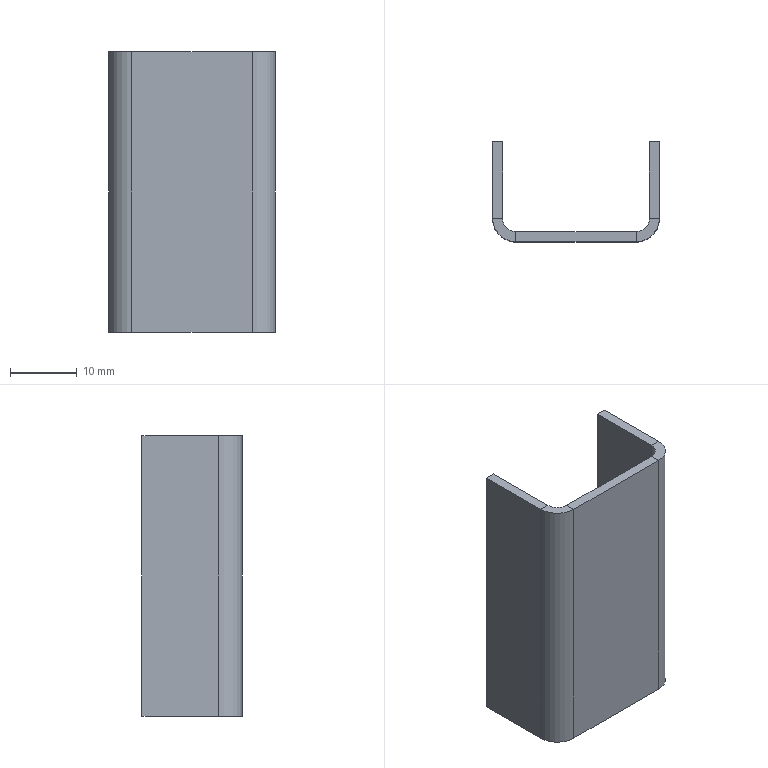Part | STEP file | Reinforcing rib 1001 | 1 solid | 22 faces | box 25 x 15 x 42 mm | volume 3127 mm3 | plane 18 | cylinder 4 | commonest cylinder face diameters 4 x2 7 x2
STEP:
#1=CARTESIAN_POINT('',(0.,0.,0.));
#2=DIRECTION('',(0.,0.,1.));
#3=DIRECTION('',(1.,0.,0.));
#4=AXIS2_PLACEMENT_3D('',#1,#2,#3);
#5=CARTESIAN_POINT('',(-12.5,3.5,21.));
#6=VERTEX_POINT('',#5);
#7=CARTESIAN_POINT('',(-11.,3.5,21.));
#8=VERTEX_POINT('',#7);
#9=CARTESIAN_POINT('',(-12.5,3.5,21.));
#10=DIRECTION('',(1.,0.,0.));
#11=VECTOR('',#10,1.);
#12=LINE('',#9,#11);
#13=CARTESIAN_POINT('',(-12.5,3.5,21.));
#14=DIRECTION('',(0.,0.,1.));
#15=DIRECTION('',(1.,0.,0.));
#16=AXIS2_PLACEMENT_3D('',#13,#14,#15);
#17=PLANE('',#16);
#18=CARTESIAN_POINT('',(0.,0.));
#19=DIRECTION('',(1.,0.));
#20=VECTOR('',#19,1.);
#21=LINE('',#18,#20);
#22=(GEOMETRIC_REPRESENTATION_CONTEXT(2)PARAMETRIC_REPRESENTATION_CONTEXT()REPRESENTATION_CONTEXT('',''));
#23=DEFINITIONAL_REPRESENTATION('',(#21),#22);
#24=PCURVE('',#17,#23);
#25=CARTESIAN_POINT('',(-9.,1.5,21.));
#26=DIRECTION('',(0.,0.,1.));
#27=DIRECTION('',(1.,0.,0.));
#28=AXIS2_PLACEMENT_3D('',#25,#26,#27);
#29=PLANE('',#28);
#30=CARTESIAN_POINT('',(-3.5,2.));
#31=DIRECTION('',(1.,0.));
#32=VECTOR('',#31,1.);
#33=LINE('',#30,#32);
#34=(GEOMETRIC_REPRESENTATION_CONTEXT(2)PARAMETRIC_REPRESENTATION_CONTEXT()REPRESENTATION_CONTEXT('',''));
#35=DEFINITIONAL_REPRESENTATION('',(#33),#34);
#36=PCURVE('',#29,#35);
#37=SURFACE_CURVE('',#12,(#24,#36),.PCURVE_S1.);
#38=EDGE_CURVE('',#6,#8,#37,.T.);
#39=ORIENTED_EDGE('',*,*,#38,.F.);
#40=CARTESIAN_POINT('',(-9.,0.,21.));
#41=VERTEX_POINT('',#40);
#42=CARTESIAN_POINT('',(-9.,3.5,21.));
#43=DIRECTION('',(0.,0.,1.));
#44=DIRECTION('',(-1.,0.,0.));
#45=AXIS2_PLACEMENT_3D('',#42,#43,#44);
#46=CIRCLE('',#45,3.5);
#47=CARTESIAN_POINT('',(3.5,0.));
#48=DIRECTION('',(-1.,0.));
#49=AXIS2_PLACEMENT_2D('',#47,#48);
#50=CIRCLE('',#49,3.5);
#51=(GEOMETRIC_REPRESENTATION_CONTEXT(2)PARAMETRIC_REPRESENTATION_CONTEXT()REPRESENTATION_CONTEXT('',''));
#52=DEFINITIONAL_REPRESENTATION('',(#50),#51);
#53=PCURVE('',#17,#52);
#54=CARTESIAN_POINT('',(-9.,3.5,21.));
#55=DIRECTION('',(0.,0.,-1.));
#56=DIRECTION('',(-1.,0.,0.));
#57=AXIS2_PLACEMENT_3D('',#54,#55,#56);
#58=CYLINDRICAL_SURFACE('',#57,3.5);
#59=CARTESIAN_POINT('',(6.283,0.));
#60=DIRECTION('',(-1.,0.));
#61=VECTOR('',#60,1.);
#62=LINE('',#59,#61);
#63=(GEOMETRIC_REPRESENTATION_CONTEXT(2)PARAMETRIC_REPRESENTATION_CONTEXT()REPRESENTATION_CONTEXT('',''));
#64=DEFINITIONAL_REPRESENTATION('',(#62),#63);
#65=PCURVE('',#58,#64);
#66=SURFACE_CURVE('',#46,(#53,#65),.PCURVE_S1.);
#67=EDGE_CURVE('',#6,#41,#66,.T.);
#68=ORIENTED_EDGE('',*,*,#67,.T.);
#69=CARTESIAN_POINT('',(-9.,1.5,21.));
#70=VERTEX_POINT('',#69);
#71=CARTESIAN_POINT('',(-9.,1.5,21.));
#72=DIRECTION('',(0.,-1.,0.));
#73=VECTOR('',#72,1.);
#74=LINE('',#71,#73);
#75=CARTESIAN_POINT('',(3.5,-2.));
#76=DIRECTION('',(0.,-1.));
#77=VECTOR('',#76,1.);
#78=LINE('',#75,#77);
#79=(GEOMETRIC_REPRESENTATION_CONTEXT(2)PARAMETRIC_REPRESENTATION_CONTEXT()REPRESENTATION_CONTEXT('',''));
#80=DEFINITIONAL_REPRESENTATION('',(#78),#79);
#81=PCURVE('',#17,#80);
#82=CARTESIAN_POINT('',(11.,3.5,21.));
#83=DIRECTION('',(0.,0.,1.));
#84=DIRECTION('',(1.,0.,0.));
#85=AXIS2_PLACEMENT_3D('',#82,#83,#84);
#86=PLANE('',#85);
#87=CARTESIAN_POINT('',(-20.,-2.));
#88=DIRECTION('',(0.,-1.));
#89=VECTOR('',#88,1.);
#90=LINE('',#87,#89);
#91=(GEOMETRIC_REPRESENTATION_CONTEXT(2)PARAMETRIC_REPRESENTATION_CONTEXT()REPRESENTATION_CONTEXT('',''));
#92=DEFINITIONAL_REPRESENTATION('',(#90),#91);
#93=PCURVE('',#86,#92);
#94=SURFACE_CURVE('',#74,(#81,#93),.PCURVE_S1.);
#95=EDGE_CURVE('',#70,#41,#94,.T.);
#96=ORIENTED_EDGE('',*,*,#95,.F.);
#97=CARTESIAN_POINT('',(-9.,3.5,21.));
#98=DIRECTION('',(0.,0.,1.));
#99=DIRECTION('',(1.,0.,0.));
#100=AXIS2_PLACEMENT_3D('',#97,#98,#99);
#101=CIRCLE('',#100,2.);
#102=CARTESIAN_POINT('',(3.5,0.));
#103=DIRECTION('',(1.,0.));
#104=AXIS2_PLACEMENT_2D('',#102,#103);
#105=CIRCLE('',#104,2.);
#106=(GEOMETRIC_REPRESENTATION_CONTEXT(2)PARAMETRIC_REPRESENTATION_CONTEXT()REPRESENTATION_CONTEXT('',''));
#107=DEFINITIONAL_REPRESENTATION('',(#105),#106);
#108=PCURVE('',#17,#107);
#109=CARTESIAN_POINT('',(-9.,3.5,21.));
#110=DIRECTION('',(0.,0.,-1.));
#111=DIRECTION('',(-1.,0.,0.));
#112=AXIS2_PLACEMENT_3D('',#109,#110,#111);
#113=CYLINDRICAL_SURFACE('',#112,2.);
#114=CARTESIAN_POINT('',(9.425,0.));
#115=DIRECTION('',(-1.,0.));
#116=VECTOR('',#115,1.);
#117=LINE('',#114,#116);
#118=(GEOMETRIC_REPRESENTATION_CONTEXT(2)PARAMETRIC_REPRESENTATION_CONTEXT()REPRESENTATION_CONTEXT('',''));
#119=DEFINITIONAL_REPRESENTATION('',(#117),#118);
#120=PCURVE('',#113,#119);
#121=SURFACE_CURVE('',#101,(#108,#120),.PCURVE_S1.);
#122=EDGE_CURVE('',#8,#70,#121,.T.);
#123=ORIENTED_EDGE('',*,*,#122,.F.);
#124=EDGE_LOOP('',(#39,#68,#96,#123));
#125=FACE_BOUND('',#124,.T.);
#126=ADVANCED_FACE('',(#125),#17,.T.);
#127=CARTESIAN_POINT('',(-12.5,15.,21.));
#128=VERTEX_POINT('',#127);
#129=CARTESIAN_POINT('',(-12.5,15.,21.));
#130=DIRECTION('',(0.,-1.,0.));
#131=VECTOR('',#130,1.);
#132=LINE('',#129,#131);
#133=CARTESIAN_POINT('',(-3.5,13.5));
#134=DIRECTION('',(0.,-1.));
#135=VECTOR('',#134,1.);
#136=LINE('',#133,#135);
#137=(GEOMETRIC_REPRESENTATION_CONTEXT(2)PARAMETRIC_REPRESENTATION_CONTEXT()REPRESENTATION_CONTEXT('',''));
#138=DEFINITIONAL_REPRESENTATION('',(#136),#137);
#139=PCURVE('',#29,#138);
#140=CARTESIAN_POINT('',(-12.5,15.,21.));
#141=DIRECTION('',(1.,0.,0.));
#142=DIRECTION('',(0.,1.,0.));
#143=AXIS2_PLACEMENT_3D('',#140,#141,#142);
#144=PLANE('',#143);
#145=CARTESIAN_POINT('',(0.,0.));
#146=DIRECTION('',(-1.,0.));
#147=VECTOR('',#146,1.);
#148=LINE('',#145,#147);
#149=(GEOMETRIC_REPRESENTATION_CONTEXT(2)PARAMETRIC_REPRESENTATION_CONTEXT()REPRESENTATION_CONTEXT('',''));
#150=DEFINITIONAL_REPRESENTATION('',(#148),#149);
#151=PCURVE('',#144,#150);
#152=SURFACE_CURVE('',#132,(#139,#151),.PCURVE_S1.);
#153=EDGE_CURVE('',#128,#6,#152,.T.);
#154=ORIENTED_EDGE('',*,*,#153,.T.);
#155=ORIENTED_EDGE('',*,*,#38,.T.);
#156=CARTESIAN_POINT('',(-11.,15.,21.));
#157=VERTEX_POINT('',#156);
#158=CARTESIAN_POINT('',(-11.,15.,21.));
#159=DIRECTION('',(0.,-1.,0.));
#160=VECTOR('',#159,1.);
#161=LINE('',#158,#160);
#162=CARTESIAN_POINT('',(-2.,13.5));
#163=DIRECTION('',(0.,-1.));
#164=VECTOR('',#163,1.);
#165=LINE('',#162,#164);
#166=(GEOMETRIC_REPRESENTATION_CONTEXT(2)PARAMETRIC_REPRESENTATION_CONTEXT()REPRESENTATION_CONTEXT('',''));
#167=DEFINITIONAL_REPRESENTATION('',(#165),#166);
#168=PCURVE('',#29,#167);
#169=CARTESIAN_POINT('',(-11.,15.,21.));
#170=DIRECTION('',(1.,0.,0.));
#171=DIRECTION('',(0.,1.,0.));
#172=AXIS2_PLACEMENT_3D('',#169,#170,#171);
#173=PLANE('',#172);
#174=CARTESIAN_POINT('',(0.,0.));
#175=DIRECTION('',(-1.,0.));
#176=VECTOR('',#175,1.);
#177=LINE('',#174,#176);
#178=(GEOMETRIC_REPRESENTATION_CONTEXT(2)PARAMETRIC_REPRESENTATION_CONTEXT()REPRESENTATION_CONTEXT('',''));
#179=DEFINITIONAL_REPRESENTATION('',(#177),#178);
#180=PCURVE('',#173,#179);
#181=SURFACE_CURVE('',#161,(#168,#180),.PCURVE_S1.);
#182=EDGE_CURVE('',#157,#8,#181,.T.);
#183=ORIENTED_EDGE('',*,*,#182,.F.);
#184=CARTESIAN_POINT('',(-12.5,15.,21.));
#185=DIRECTION('',(1.,0.,0.));
#186=VECTOR('',#185,1.);
#187=LINE('',#184,#186);
#188=CARTESIAN_POINT('',(-3.5,13.5));
#189=DIRECTION('',(1.,0.));
#190=VECTOR('',#189,1.);
#191=LINE('',#188,#190);
#192=(GEOMETRIC_REPRESENTATION_CONTEXT(2)PARAMETRIC_REPRESENTATION_CONTEXT()REPRESENTATION_CONTEXT('',''));
#193=DEFINITIONAL_REPRESENTATION('',(#191),#192);
#194=PCURVE('',#29,#193);
#195=CARTESIAN_POINT('',(-12.5,15.,21.));
#196=DIRECTION('',(0.,1.,0.));
#197=DIRECTION('',(0.,0.,1.));
#198=AXIS2_PLACEMENT_3D('',#195,#196,#197);
#199=PLANE('',#198);
#200=CARTESIAN_POINT('',(0.,0.));
#201=DIRECTION('',(0.,1.));
#202=VECTOR('',#201,1.);
#203=LINE('',#200,#202);
#204=(GEOMETRIC_REPRESENTATION_CONTEXT(2)PARAMETRIC_REPRESENTATION_CONTEXT()REPRESENTATION_CONTEXT('',''));
#205=DEFINITIONAL_REPRESENTATION('',(#203),#204);
#206=PCURVE('',#199,#205);
#207=SURFACE_CURVE('',#187,(#194,#206),.PCURVE_S1.);
#208=EDGE_CURVE('',#128,#157,#207,.T.);
#209=ORIENTED_EDGE('',*,*,#208,.F.);
#210=EDGE_LOOP('',(#154,#155,#183,#209));
#211=FACE_BOUND('',#210,.T.);
#212=ADVANCED_FACE('',(#211),#29,.T.);
#213=CARTESIAN_POINT('',(-9.,0.,-21.));
#214=VERTEX_POINT('',#213);
#215=CARTESIAN_POINT('',(-9.,1.5,-21.));
#216=VERTEX_POINT('',#215);
#217=CARTESIAN_POINT('',(-9.,0.,-21.));
#218=DIRECTION('',(0.,1.,0.));
#219=VECTOR('',#218,1.);
#220=LINE('',#217,#219);
#221=CARTESIAN_POINT('',(-9.,0.,-21.));
#222=DIRECTION('',(0.,0.,-1.));
#223=DIRECTION('',(-1.,0.,0.));
#224=AXIS2_PLACEMENT_3D('',#221,#222,#223);
#225=PLANE('',#224);
#226=CARTESIAN_POINT('',(0.,0.));
#227=DIRECTION('',(0.,1.));
#228=VECTOR('',#227,1.);
#229=LINE('',#226,#228);
#230=(GEOMETRIC_REPRESENTATION_CONTEXT(2)PARAMETRIC_REPRESENTATION_CONTEXT()REPRESENTATION_CONTEXT('',''));
#231=DEFINITIONAL_REPRESENTATION('',(#229),#230);
#232=PCURVE('',#225,#231);
#233=CARTESIAN_POINT('',(-11.,3.5,-21.));
#234=DIRECTION('',(0.,0.,-1.));
#235=DIRECTION('',(-1.,0.,0.));
#236=AXIS2_PLACEMENT_3D('',#233,#234,#235);
#237=PLANE('',#236);
#238=CARTESIAN_POINT('',(-2.,-3.5));
#239=DIRECTION('',(0.,1.));
#240=VECTOR('',#239,1.);
#241=LINE('',#238,#240);
#242=(GEOMETRIC_REPRESENTATION_CONTEXT(2)PARAMETRIC_REPRESENTATION_CONTEXT()REPRESENTATION_CONTEXT('',''));
#243=DEFINITIONAL_REPRESENTATION('',(#241),#242);
#244=PCURVE('',#237,#243);
#245=SURFACE_CURVE('',#220,(#232,#244),.PCURVE_S1.);
#246=EDGE_CURVE('',#214,#216,#245,.T.);
#247=ORIENTED_EDGE('',*,*,#246,.F.);
#248=CARTESIAN_POINT('',(-12.5,3.5,-21.));
#249=VERTEX_POINT('',#248);
#250=CARTESIAN_POINT('',(-9.,3.5,-21.));
#251=DIRECTION('',(0.,0.,1.));
#252=DIRECTION('',(-1.,0.,0.));
#253=AXIS2_PLACEMENT_3D('',#250,#251,#252);
#254=CIRCLE('',#253,3.5);
#255=CARTESIAN_POINT('',(3.5,3.5));
#256=CARTESIAN_POINT('',(3.5,-2.562));
#257=CARTESIAN_POINT('',(-1.75,0.4689));
#258=CARTESIAN_POINT('',(-7.,3.5));
#259=CARTESIAN_POINT('',(-1.75,6.531));
#260=CARTESIAN_POINT('',(3.5,9.562));
#261=CARTESIAN_POINT('',(3.5,3.5));
#262=(BOUNDED_CURVE()B_SPLINE_CURVE(2,(#255,#256,#257,#258,#259,#260,#261),.UNSPECIFIED.,.T.,.F.)B_SPLINE_CURVE_WITH_KNOTS((1,2,2,2,2,1),(-2.094,0.,2.094,4.189,6.283,8.378),.UNSPECIFIED.)CURVE()GEOMETRIC_REPRESENTATION_ITEM()RATIONAL_B_SPLINE_CURVE((1.,0.5,1.,0.5,1.,0.5,1.))REPRESENTATION_ITEM(''));
#263=(GEOMETRIC_REPRESENTATION_CONTEXT(2)PARAMETRIC_REPRESENTATION_CONTEXT()REPRESENTATION_CONTEXT('',''));
#264=DEFINITIONAL_REPRESENTATION('',(#262),#263);
#265=PCURVE('',#225,#264);
#266=CARTESIAN_POINT('',(6.283,42.));
#267=DIRECTION('',(-1.,0.));
#268=VECTOR('',#267,1.);
#269=LINE('',#266,#268);
#270=(GEOMETRIC_REPRESENTATION_CONTEXT(2)PARAMETRIC_REPRESENTATION_CONTEXT()REPRESENTATION_CONTEXT('',''));
#271=DEFINITIONAL_REPRESENTATION('',(#269),#270);
#272=PCURVE('',#58,#271);
#273=SURFACE_CURVE('',#254,(#265,#272),.PCURVE_S1.);
#274=EDGE_CURVE('',#249,#214,#273,.T.);
#275=ORIENTED_EDGE('',*,*,#274,.F.);
#276=CARTESIAN_POINT('',(-11.,3.5,-21.));
#277=VERTEX_POINT('',#276);
#278=CARTESIAN_POINT('',(-11.,3.5,-21.));
#279=DIRECTION('',(-1.,0.,0.));
#280=VECTOR('',#279,1.);
#281=LINE('',#278,#280);
#282=CARTESIAN_POINT('',(2.,3.5));
#283=DIRECTION('',(1.,0.));
#284=VECTOR('',#283,1.);
#285=LINE('',#282,#284);
#286=(GEOMETRIC_REPRESENTATION_CONTEXT(2)PARAMETRIC_REPRESENTATION_CONTEXT()REPRESENTATION_CONTEXT('',''));
#287=DEFINITIONAL_REPRESENTATION('',(#285),#286);
#288=PCURVE('',#225,#287);
#289=CARTESIAN_POINT('',(9.,3.5,-21.));
#290=DIRECTION('',(0.,0.,1.));
#291=DIRECTION('',(1.,0.,0.));
#292=AXIS2_PLACEMENT_3D('',#289,#290,#291);
#293=PLANE('',#292);
#294=CARTESIAN_POINT('',(-20.,0.));
#295=DIRECTION('',(-1.,0.));
#296=VECTOR('',#295,1.);
#297=LINE('',#294,#296);
#298=(GEOMETRIC_REPRESENTATION_CONTEXT(2)PARAMETRIC_REPRESENTATION_CONTEXT()REPRESENTATION_CONTEXT('',''));
#299=DEFINITIONAL_REPRESENTATION('',(#297),#298);
#300=PCURVE('',#293,#299);
#301=SURFACE_CURVE('',#281,(#288,#300),.PCURVE_S1.);
#302=EDGE_CURVE('',#277,#249,#301,.T.);
#303=ORIENTED_EDGE('',*,*,#302,.F.);
#304=CARTESIAN_POINT('',(-9.,3.5,-21.));
#305=DIRECTION('',(0.,0.,1.));
#306=DIRECTION('',(1.,0.,0.));
#307=AXIS2_PLACEMENT_3D('',#304,#305,#306);
#308=CIRCLE('',#307,2.);
#309=CARTESIAN_POINT('',(-2.,3.5));
#310=CARTESIAN_POINT('',(-2.,6.964));
#311=CARTESIAN_POINT('',(1.,5.232));
#312=CARTESIAN_POINT('',(4.,3.5));
#313=CARTESIAN_POINT('',(1.,1.768));
#314=CARTESIAN_POINT('',(-2.,0.0359));
#315=CARTESIAN_POINT('',(-2.,3.5));
#316=(BOUNDED_CURVE()B_SPLINE_CURVE(2,(#309,#310,#311,#312,#313,#314,#315),.UNSPECIFIED.,.T.,.F.)B_SPLINE_CURVE_WITH_KNOTS((1,2,2,2,2,1),(-2.094,0.,2.094,4.189,6.283,8.378),.UNSPECIFIED.)CURVE()GEOMETRIC_REPRESENTATION_ITEM()RATIONAL_B_SPLINE_CURVE((1.,0.5,1.,0.5,1.,0.5,1.))REPRESENTATION_ITEM(''));
#317=(GEOMETRIC_REPRESENTATION_CONTEXT(2)PARAMETRIC_REPRESENTATION_CONTEXT()REPRESENTATION_CONTEXT('',''));
#318=DEFINITIONAL_REPRESENTATION('',(#316),#317);
#319=PCURVE('',#225,#318);
#320=CARTESIAN_POINT('',(9.425,42.));
#321=DIRECTION('',(-1.,0.));
#322=VECTOR('',#321,1.);
#323=LINE('',#320,#322);
#324=(GEOMETRIC_REPRESENTATION_CONTEXT(2)PARAMETRIC_REPRESENTATION_CONTEXT()REPRESENTATION_CONTEXT('',''));
#325=DEFINITIONAL_REPRESENTATION('',(#323),#324);
#326=PCURVE('',#113,#325);
#327=SURFACE_CURVE('',#308,(#319,#326),.PCURVE_S1.);
#328=EDGE_CURVE('',#277,#216,#327,.T.);
#329=ORIENTED_EDGE('',*,*,#328,.T.);
#330=EDGE_LOOP('',(#247,#275,#303,#329));
#331=FACE_BOUND('',#330,.T.);
#332=ADVANCED_FACE('',(#331),#225,.T.);
#333=CARTESIAN_POINT('',(9.,0.,-21.));
#334=VERTEX_POINT('',#333);
#335=CARTESIAN_POINT('',(-12.5,0.,-21.));
#336=DIRECTION('',(1.,0.,0.));
#337=VECTOR('',#336,1.);
#338=LINE('',#335,#337);
#339=CARTESIAN_POINT('',(1.5,-3.5));
#340=DIRECTION('',(-1.,0.));
#341=VECTOR('',#340,1.);
#342=LINE('',#339,#341);
#343=(GEOMETRIC_REPRESENTATION_CONTEXT(2)PARAMETRIC_REPRESENTATION_CONTEXT()REPRESENTATION_CONTEXT('',''));
#344=DEFINITIONAL_REPRESENTATION('',(#342),#343);
#345=PCURVE('',#237,#344);
#346=CARTESIAN_POINT('',(-12.5,0.,21.));
#347=DIRECTION('',(0.,1.,0.));
#348=DIRECTION('',(0.,0.,1.));
#349=AXIS2_PLACEMENT_3D('',#346,#347,#348);
#350=PLANE('',#349);
#351=CARTESIAN_POINT('',(-42.,0.));
#352=DIRECTION('',(0.,1.));
#353=VECTOR('',#352,1.);
#354=LINE('',#351,#353);
#355=(GEOMETRIC_REPRESENTATION_CONTEXT(2)PARAMETRIC_REPRESENTATION_CONTEXT()REPRESENTATION_CONTEXT('',''));
#356=DEFINITIONAL_REPRESENTATION('',(#354),#355);
#357=PCURVE('',#350,#356);
#358=SURFACE_CURVE('',#338,(#345,#357),.PCURVE_S1.);
#359=EDGE_CURVE('',#214,#334,#358,.T.);
#360=ORIENTED_EDGE('',*,*,#359,.F.);
#361=ORIENTED_EDGE('',*,*,#246,.T.);
#362=CARTESIAN_POINT('',(9.,1.5,-21.));
#363=VERTEX_POINT('',#362);
#364=CARTESIAN_POINT('',(-12.5,1.5,-21.));
#365=DIRECTION('',(1.,0.,0.));
#366=VECTOR('',#365,1.);
#367=LINE('',#364,#366);
#368=CARTESIAN_POINT('',(1.5,-2.));
#369=DIRECTION('',(-1.,0.));
#370=VECTOR('',#369,1.);
#371=LINE('',#368,#370);
#372=(GEOMETRIC_REPRESENTATION_CONTEXT(2)PARAMETRIC_REPRESENTATION_CONTEXT()REPRESENTATION_CONTEXT('',''));
#373=DEFINITIONAL_REPRESENTATION('',(#371),#372);
#374=PCURVE('',#237,#373);
#375=CARTESIAN_POINT('',(-12.5,1.5,21.));
#376=DIRECTION('',(0.,1.,0.));
#377=DIRECTION('',(0.,0.,1.));
#378=AXIS2_PLACEMENT_3D('',#375,#376,#377);
#379=PLANE('',#378);
#380=CARTESIAN_POINT('',(-42.,0.));
#381=DIRECTION('',(0.,1.));
#382=VECTOR('',#381,1.);
#383=LINE('',#380,#382);
#384=(GEOMETRIC_REPRESENTATION_CONTEXT(2)PARAMETRIC_REPRESENTATION_CONTEXT()REPRESENTATION_CONTEXT('',''));
#385=DEFINITIONAL_REPRESENTATION('',(#383),#384);
#386=PCURVE('',#379,#385);
#387=SURFACE_CURVE('',#367,(#374,#386),.PCURVE_S1.);
#388=EDGE_CURVE('',#216,#363,#387,.T.);
#389=ORIENTED_EDGE('',*,*,#388,.T.);
#390=CARTESIAN_POINT('',(9.,1.5,-21.));
#391=DIRECTION('',(0.,-1.,0.));
#392=VECTOR('',#391,1.);
#393=LINE('',#390,#392);
#394=CARTESIAN_POINT('',(-20.,-2.));
#395=DIRECTION('',(0.,-1.));
#396=VECTOR('',#395,1.);
#397=LINE('',#394,#396);
#398=(GEOMETRIC_REPRESENTATION_CONTEXT(2)PARAMETRIC_REPRESENTATION_CONTEXT()REPRESENTATION_CONTEXT('',''));
#399=DEFINITIONAL_REPRESENTATION('',(#397),#398);
#400=PCURVE('',#237,#399);
#401=CARTESIAN_POINT('',(12.5,3.5,-21.));
#402=DIRECTION('',(0.,0.,-1.));
#403=DIRECTION('',(-1.,0.,0.));
#404=AXIS2_PLACEMENT_3D('',#401,#402,#403);
#405=PLANE('',#404);
#406=CARTESIAN_POINT('',(3.5,-2.));
#407=DIRECTION('',(0.,-1.));
#408=VECTOR('',#407,1.);
#409=LINE('',#406,#408);
#410=(GEOMETRIC_REPRESENTATION_CONTEXT(2)PARAMETRIC_REPRESENTATION_CONTEXT()REPRESENTATION_CONTEXT('',''));
#411=DEFINITIONAL_REPRESENTATION('',(#409),#410);
#412=PCURVE('',#405,#411);
#413=SURFACE_CURVE('',#393,(#400,#412),.PCURVE_S1.);
#414=EDGE_CURVE('',#363,#334,#413,.T.);
#415=ORIENTED_EDGE('',*,*,#414,.T.);
#416=EDGE_LOOP('',(#360,#361,#389,#415));
#417=FACE_BOUND('',#416,.T.);
#418=ADVANCED_FACE('',(#417),#237,.T.);
#419=CARTESIAN_POINT('',(9.,0.,21.));
#420=VERTEX_POINT('',#419);
#421=CARTESIAN_POINT('',(9.,1.5,21.));
#422=VERTEX_POINT('',#421);
#423=CARTESIAN_POINT('',(9.,0.,21.));
#424=DIRECTION('',(0.,1.,0.));
#425=VECTOR('',#424,1.);
#426=LINE('',#423,#425);
#427=CARTESIAN_POINT('',(9.,0.,21.));
#428=DIRECTION('',(0.,0.,1.));
#429=DIRECTION('',(1.,0.,0.));
#430=AXIS2_PLACEMENT_3D('',#427,#428,#429);
#431=PLANE('',#430);
#432=CARTESIAN_POINT('',(0.,0.));
#433=DIRECTION('',(0.,1.));
#434=VECTOR('',#433,1.);
#435=LINE('',#432,#434);
#436=(GEOMETRIC_REPRESENTATION_CONTEXT(2)PARAMETRIC_REPRESENTATION_CONTEXT()REPRESENTATION_CONTEXT('',''));
#437=DEFINITIONAL_REPRESENTATION('',(#435),#436);
#438=PCURVE('',#431,#437);
#439=CARTESIAN_POINT('',(-2.,-3.5));
#440=DIRECTION('',(0.,1.));
#441=VECTOR('',#440,1.);
#442=LINE('',#439,#441);
#443=(GEOMETRIC_REPRESENTATION_CONTEXT(2)PARAMETRIC_REPRESENTATION_CONTEXT()REPRESENTATION_CONTEXT('',''));
#444=DEFINITIONAL_REPRESENTATION('',(#442),#443);
#445=PCURVE('',#86,#444);
#446=SURFACE_CURVE('',#426,(#438,#445),.PCURVE_S1.);
#447=EDGE_CURVE('',#420,#422,#446,.T.);
#448=ORIENTED_EDGE('',*,*,#447,.F.);
#449=CARTESIAN_POINT('',(12.5,3.5,21.));
#450=VERTEX_POINT('',#449);
#451=CARTESIAN_POINT('',(9.,3.5,21.));
#452=DIRECTION('',(0.,0.,1.));
#453=DIRECTION('',(-1.,0.,0.));
#454=AXIS2_PLACEMENT_3D('',#451,#452,#453);
#455=CIRCLE('',#454,3.5);
#456=CARTESIAN_POINT('',(0.,3.5));
#457=DIRECTION('',(-1.,0.));
#458=AXIS2_PLACEMENT_2D('',#456,#457);
#459=CIRCLE('',#458,3.5);
#460=(GEOMETRIC_REPRESENTATION_CONTEXT(2)PARAMETRIC_REPRESENTATION_CONTEXT()REPRESENTATION_CONTEXT('',''));
#461=DEFINITIONAL_REPRESENTATION('',(#459),#460);
#462=PCURVE('',#431,#461);
#463=CARTESIAN_POINT('',(9.,3.5,21.));
#464=DIRECTION('',(0.,0.,-1.));
#465=DIRECTION('',(-1.,0.,0.));
#466=AXIS2_PLACEMENT_3D('',#463,#464,#465);
#467=CYLINDRICAL_SURFACE('',#466,3.5);
#468=CARTESIAN_POINT('',(6.283,0.));
#469=DIRECTION('',(-1.,0.));
#470=VECTOR('',#469,1.);
#471=LINE('',#468,#470);
#472=(GEOMETRIC_REPRESENTATION_CONTEXT(2)PARAMETRIC_REPRESENTATION_CONTEXT()REPRESENTATION_CONTEXT('',''));
#473=DEFINITIONAL_REPRESENTATION('',(#471),#472);
#474=PCURVE('',#467,#473);
#475=SURFACE_CURVE('',#455,(#462,#474),.PCURVE_S1.);
#476=EDGE_CURVE('',#420,#450,#475,.T.);
#477=ORIENTED_EDGE('',*,*,#476,.T.);
#478=CARTESIAN_POINT('',(11.,3.5,21.));
#479=VERTEX_POINT('',#478);
#480=CARTESIAN_POINT('',(11.,3.5,21.));
#481=DIRECTION('',(1.,0.,0.));
#482=VECTOR('',#481,1.);
#483=LINE('',#480,#482);
#484=CARTESIAN_POINT('',(2.,3.5));
#485=DIRECTION('',(1.,0.));
#486=VECTOR('',#485,1.);
#487=LINE('',#484,#486);
#488=(GEOMETRIC_REPRESENTATION_CONTEXT(2)PARAMETRIC_REPRESENTATION_CONTEXT()REPRESENTATION_CONTEXT('',''));
#489=DEFINITIONAL_REPRESENTATION('',(#487),#488);
#490=PCURVE('',#431,#489);
#491=CARTESIAN_POINT('',(9.,3.5,21.));
#492=DIRECTION('',(0.,0.,1.));
#493=DIRECTION('',(1.,0.,0.));
#494=AXIS2_PLACEMENT_3D('',#491,#492,#493);
#495=PLANE('',#494);
#496=CARTESIAN_POINT('',(2.,0.));
#497=DIRECTION('',(1.,0.));
#498=VECTOR('',#497,1.);
#499=LINE('',#496,#498);
#500=(GEOMETRIC_REPRESENTATION_CONTEXT(2)PARAMETRIC_REPRESENTATION_CONTEXT()REPRESENTATION_CONTEXT('',''));
#501=DEFINITIONAL_REPRESENTATION('',(#499),#500);
#502=PCURVE('',#495,#501);
#503=SURFACE_CURVE('',#483,(#490,#502),.PCURVE_S1.);
#504=EDGE_CURVE('',#479,#450,#503,.T.);
#505=ORIENTED_EDGE('',*,*,#504,.F.);
#506=CARTESIAN_POINT('',(9.,3.5,21.));
#507=DIRECTION('',(0.,0.,1.));
#508=DIRECTION('',(1.,0.,0.));
#509=AXIS2_PLACEMENT_3D('',#506,#507,#508);
#510=CIRCLE('',#509,2.);
#511=CARTESIAN_POINT('',(0.,3.5));
#512=DIRECTION('',(1.,0.));
#513=AXIS2_PLACEMENT_2D('',#511,#512);
#514=CIRCLE('',#513,2.);
#515=(GEOMETRIC_REPRESENTATION_CONTEXT(2)PARAMETRIC_REPRESENTATION_CONTEXT()REPRESENTATION_CONTEXT('',''));
#516=DEFINITIONAL_REPRESENTATION('',(#514),#515);
#517=PCURVE('',#431,#516);
#518=CARTESIAN_POINT('',(9.,3.5,21.));
#519=DIRECTION('',(0.,0.,-1.));
#520=DIRECTION('',(-1.,0.,0.));
#521=AXIS2_PLACEMENT_3D('',#518,#519,#520);
#522=CYLINDRICAL_SURFACE('',#521,2.);
#523=CARTESIAN_POINT('',(9.425,0.));
#524=DIRECTION('',(-1.,0.));
#525=VECTOR('',#524,1.);
#526=LINE('',#523,#525);
#527=(GEOMETRIC_REPRESENTATION_CONTEXT(2)PARAMETRIC_REPRESENTATION_CONTEXT()REPRESENTATION_CONTEXT('',''));
#528=DEFINITIONAL_REPRESENTATION('',(#526),#527);
#529=PCURVE('',#522,#528);
#530=SURFACE_CURVE('',#510,(#517,#529),.PCURVE_S1.);
#531=EDGE_CURVE('',#422,#479,#530,.T.);
#532=ORIENTED_EDGE('',*,*,#531,.F.);
#533=EDGE_LOOP('',(#448,#477,#505,#532));
#534=FACE_BOUND('',#533,.T.);
#535=ADVANCED_FACE('',(#534),#431,.T.);
#536=CARTESIAN_POINT('',(-12.5,0.,21.));
#537=DIRECTION('',(1.,0.,0.));
#538=VECTOR('',#537,1.);
#539=LINE('',#536,#538);
#540=CARTESIAN_POINT('',(-23.5,-3.5));
#541=DIRECTION('',(1.,0.));
#542=VECTOR('',#541,1.);
#543=LINE('',#540,#542);
#544=(GEOMETRIC_REPRESENTATION_CONTEXT(2)PARAMETRIC_REPRESENTATION_CONTEXT()REPRESENTATION_CONTEXT('',''));
#545=DEFINITIONAL_REPRESENTATION('',(#543),#544);
#546=PCURVE('',#86,#545);
#547=CARTESIAN_POINT('',(0.,0.));
#548=DIRECTION('',(0.,1.));
#549=VECTOR('',#548,1.);
#550=LINE('',#547,#549);
#551=(GEOMETRIC_REPRESENTATION_CONTEXT(2)PARAMETRIC_REPRESENTATION_CONTEXT()REPRESENTATION_CONTEXT('',''));
#552=DEFINITIONAL_REPRESENTATION('',(#550),#551);
#553=PCURVE('',#350,#552);
#554=SURFACE_CURVE('',#539,(#546,#553),.PCURVE_S1.);
#555=EDGE_CURVE('',#41,#420,#554,.T.);
#556=ORIENTED_EDGE('',*,*,#555,.T.);
#557=ORIENTED_EDGE('',*,*,#447,.T.);
#558=CARTESIAN_POINT('',(-12.5,1.5,21.));
#559=DIRECTION('',(1.,0.,0.));
#560=VECTOR('',#559,1.);
#561=LINE('',#558,#560);
#562=CARTESIAN_POINT('',(-23.5,-2.));
#563=DIRECTION('',(1.,0.));
#564=VECTOR('',#563,1.);
#565=LINE('',#562,#564);
#566=(GEOMETRIC_REPRESENTATION_CONTEXT(2)PARAMETRIC_REPRESENTATION_CONTEXT()REPRESENTATION_CONTEXT('',''));
#567=DEFINITIONAL_REPRESENTATION('',(#565),#566);
#568=PCURVE('',#86,#567);
#569=CARTESIAN_POINT('',(0.,0.));
#570=DIRECTION('',(0.,1.));
#571=VECTOR('',#570,1.);
#572=LINE('',#569,#571);
#573=(GEOMETRIC_REPRESENTATION_CONTEXT(2)PARAMETRIC_REPRESENTATION_CONTEXT()REPRESENTATION_CONTEXT('',''));
#574=DEFINITIONAL_REPRESENTATION('',(#572),#573);
#575=PCURVE('',#379,#574);
#576=SURFACE_CURVE('',#561,(#568,#575),.PCURVE_S1.);
#577=EDGE_CURVE('',#70,#422,#576,.T.);
#578=ORIENTED_EDGE('',*,*,#577,.F.);
#579=ORIENTED_EDGE('',*,*,#95,.T.);
#580=EDGE_LOOP('',(#556,#557,#578,#579));
#581=FACE_BOUND('',#580,.T.);
#582=ADVANCED_FACE('',(#581),#86,.T.);
#583=CARTESIAN_POINT('',(12.5,3.5,-21.));
#584=VERTEX_POINT('',#583);
#585=CARTESIAN_POINT('',(11.,3.5,-21.));
#586=VERTEX_POINT('',#585);
#587=CARTESIAN_POINT('',(12.5,3.5,-21.));
#588=DIRECTION('',(-1.,0.,0.));
#589=VECTOR('',#588,1.);
#590=LINE('',#587,#589);
#591=CARTESIAN_POINT('',(0.,0.));
#592=DIRECTION('',(1.,0.));
#593=VECTOR('',#592,1.);
#594=LINE('',#591,#593);
#595=(GEOMETRIC_REPRESENTATION_CONTEXT(2)PARAMETRIC_REPRESENTATION_CONTEXT()REPRESENTATION_CONTEXT('',''));
#596=DEFINITIONAL_REPRESENTATION('',(#594),#595);
#597=PCURVE('',#405,#596);
#598=CARTESIAN_POINT('',(9.,1.5,-21.));
#599=DIRECTION('',(0.,0.,-1.));
#600=DIRECTION('',(-1.,0.,0.));
#601=AXIS2_PLACEMENT_3D('',#598,#599,#600);
#602=PLANE('',#601);
#603=CARTESIAN_POINT('',(-3.5,2.));
#604=DIRECTION('',(1.,0.));
#605=VECTOR('',#604,1.);
#606=LINE('',#603,#605);
#607=(GEOMETRIC_REPRESENTATION_CONTEXT(2)PARAMETRIC_REPRESENTATION_CONTEXT()REPRESENTATION_CONTEXT('',''));
#608=DEFINITIONAL_REPRESENTATION('',(#606),#607);
#609=PCURVE('',#602,#608);
#610=SURFACE_CURVE('',#590,(#597,#609),.PCURVE_S1.);
#611=EDGE_CURVE('',#584,#586,#610,.T.);
#612=ORIENTED_EDGE('',*,*,#611,.F.);
#613=CARTESIAN_POINT('',(9.,3.5,-21.));
#614=DIRECTION('',(0.,0.,1.));
#615=DIRECTION('',(-1.,0.,0.));
#616=AXIS2_PLACEMENT_3D('',#613,#614,#615);
#617=CIRCLE('',#616,3.5);
#618=CARTESIAN_POINT('',(7.,0.));
#619=CARTESIAN_POINT('',(7.,-6.062));
#620=CARTESIAN_POINT('',(1.75,-3.031));
#621=CARTESIAN_POINT('',(-3.5,0.));
#622=CARTESIAN_POINT('',(1.75,3.031));
#623=CARTESIAN_POINT('',(7.,6.062));
#624=CARTESIAN_POINT('',(7.,0.));
#625=(BOUNDED_CURVE()B_SPLINE_CURVE(2,(#618,#619,#620,#621,#622,#623,#624),.UNSPECIFIED.,.T.,.F.)B_SPLINE_CURVE_WITH_KNOTS((1,2,2,2,2,1),(-2.094,0.,2.094,4.189,6.283,8.378),.UNSPECIFIED.)CURVE()GEOMETRIC_REPRESENTATION_ITEM()RATIONAL_B_SPLINE_CURVE((1.,0.5,1.,0.5,1.,0.5,1.))REPRESENTATION_ITEM(''));
#626=(GEOMETRIC_REPRESENTATION_CONTEXT(2)PARAMETRIC_REPRESENTATION_CONTEXT()REPRESENTATION_CONTEXT('',''));
#627=DEFINITIONAL_REPRESENTATION('',(#625),#626);
#628=PCURVE('',#405,#627);
#629=CARTESIAN_POINT('',(6.283,42.));
#630=DIRECTION('',(-1.,0.));
#631=VECTOR('',#630,1.);
#632=LINE('',#629,#631);
#633=(GEOMETRIC_REPRESENTATION_CONTEXT(2)PARAMETRIC_REPRESENTATION_CONTEXT()REPRESENTATION_CONTEXT('',''));
#634=DEFINITIONAL_REPRESENTATION('',(#632),#633);
#635=PCURVE('',#467,#634);
#636=SURFACE_CURVE('',#617,(#628,#635),.PCURVE_S1.);
#637=EDGE_CURVE('',#334,#584,#636,.T.);
#638=ORIENTED_EDGE('',*,*,#637,.F.);
#639=ORIENTED_EDGE('',*,*,#414,.F.);
#640=CARTESIAN_POINT('',(9.,3.5,-21.));
#641=DIRECTION('',(0.,0.,1.));
#642=DIRECTION('',(1.,0.,0.));
#643=AXIS2_PLACEMENT_3D('',#640,#641,#642);
#644=CIRCLE('',#643,2.);
#645=CARTESIAN_POINT('',(1.5,0.));
#646=CARTESIAN_POINT('',(1.5,3.464));
#647=CARTESIAN_POINT('',(4.5,1.732));
#648=CARTESIAN_POINT('',(7.5,0.));
#649=CARTESIAN_POINT('',(4.5,-1.732));
#650=CARTESIAN_POINT('',(1.5,-3.464));
#651=CARTESIAN_POINT('',(1.5,0.));
#652=(BOUNDED_CURVE()B_SPLINE_CURVE(2,(#645,#646,#647,#648,#649,#650,#651),.UNSPECIFIED.,.T.,.F.)B_SPLINE_CURVE_WITH_KNOTS((1,2,2,2,2,1),(-2.094,0.,2.094,4.189,6.283,8.378),.UNSPECIFIED.)CURVE()GEOMETRIC_REPRESENTATION_ITEM()RATIONAL_B_SPLINE_CURVE((1.,0.5,1.,0.5,1.,0.5,1.))REPRESENTATION_ITEM(''));
#653=(GEOMETRIC_REPRESENTATION_CONTEXT(2)PARAMETRIC_REPRESENTATION_CONTEXT()REPRESENTATION_CONTEXT('',''));
#654=DEFINITIONAL_REPRESENTATION('',(#652),#653);
#655=PCURVE('',#405,#654);
#656=CARTESIAN_POINT('',(9.425,42.));
#657=DIRECTION('',(-1.,0.));
#658=VECTOR('',#657,1.);
#659=LINE('',#656,#658);
#660=(GEOMETRIC_REPRESENTATION_CONTEXT(2)PARAMETRIC_REPRESENTATION_CONTEXT()REPRESENTATION_CONTEXT('',''));
#661=DEFINITIONAL_REPRESENTATION('',(#659),#660);
#662=PCURVE('',#522,#661);
#663=SURFACE_CURVE('',#644,(#655,#662),.PCURVE_S1.);
#664=EDGE_CURVE('',#363,#586,#663,.T.);
#665=ORIENTED_EDGE('',*,*,#664,.T.);
#666=EDGE_LOOP('',(#612,#638,#639,#665));
#667=FACE_BOUND('',#666,.T.);
#668=ADVANCED_FACE('',(#667),#405,.T.);
#669=CARTESIAN_POINT('',(12.5,15.,-21.));
#670=VERTEX_POINT('',#669);
#671=CARTESIAN_POINT('',(12.5,0.,-21.));
#672=DIRECTION('',(0.,1.,0.));
#673=VECTOR('',#672,1.);
#674=LINE('',#671,#673);
#675=CARTESIAN_POINT('',(-3.5,-1.5));
#676=DIRECTION('',(0.,1.));
#677=VECTOR('',#676,1.);
#678=LINE('',#675,#677);
#679=(GEOMETRIC_REPRESENTATION_CONTEXT(2)PARAMETRIC_REPRESENTATION_CONTEXT()REPRESENTATION_CONTEXT('',''));
#680=DEFINITIONAL_REPRESENTATION('',(#678),#679);
#681=PCURVE('',#602,#680);
#682=CARTESIAN_POINT('',(12.5,0.,21.));
#683=DIRECTION('',(-1.,0.,0.));
#684=DIRECTION('',(0.,-1.,0.));
#685=AXIS2_PLACEMENT_3D('',#682,#683,#684);
#686=PLANE('',#685);
#687=CARTESIAN_POINT('',(0.,-42.));
#688=DIRECTION('',(-1.,0.));
#689=VECTOR('',#688,1.);
#690=LINE('',#687,#689);
#691=(GEOMETRIC_REPRESENTATION_CONTEXT(2)PARAMETRIC_REPRESENTATION_CONTEXT()REPRESENTATION_CONTEXT('',''));
#692=DEFINITIONAL_REPRESENTATION('',(#690),#691);
#693=PCURVE('',#686,#692);
#694=SURFACE_CURVE('',#674,(#681,#693),.PCURVE_S1.);
#695=EDGE_CURVE('',#584,#670,#694,.T.);
#696=ORIENTED_EDGE('',*,*,#695,.F.);
#697=ORIENTED_EDGE('',*,*,#611,.T.);
#698=CARTESIAN_POINT('',(11.,15.,-21.));
#699=VERTEX_POINT('',#698);
#700=CARTESIAN_POINT('',(11.,0.,-21.));
#701=DIRECTION('',(0.,1.,0.));
#702=VECTOR('',#701,1.);
#703=LINE('',#700,#702);
#704=CARTESIAN_POINT('',(-2.,-1.5));
#705=DIRECTION('',(0.,1.));
#706=VECTOR('',#705,1.);
#707=LINE('',#704,#706);
#708=(GEOMETRIC_REPRESENTATION_CONTEXT(2)PARAMETRIC_REPRESENTATION_CONTEXT()REPRESENTATION_CONTEXT('',''));
#709=DEFINITIONAL_REPRESENTATION('',(#707),#708);
#710=PCURVE('',#602,#709);
#711=CARTESIAN_POINT('',(11.,0.,21.));
#712=DIRECTION('',(-1.,0.,0.));
#713=DIRECTION('',(0.,-1.,0.));
#714=AXIS2_PLACEMENT_3D('',#711,#712,#713);
#715=PLANE('',#714);
#716=CARTESIAN_POINT('',(0.,-42.));
#717=DIRECTION('',(-1.,0.));
#718=VECTOR('',#717,1.);
#719=LINE('',#716,#718);
#720=(GEOMETRIC_REPRESENTATION_CONTEXT(2)PARAMETRIC_REPRESENTATION_CONTEXT()REPRESENTATION_CONTEXT('',''));
#721=DEFINITIONAL_REPRESENTATION('',(#719),#720);
#722=PCURVE('',#715,#721);
#723=SURFACE_CURVE('',#703,(#710,#722),.PCURVE_S1.);
#724=EDGE_CURVE('',#586,#699,#723,.T.);
#725=ORIENTED_EDGE('',*,*,#724,.T.);
#726=CARTESIAN_POINT('',(11.,15.,-21.));
#727=DIRECTION('',(1.,0.,0.));
#728=VECTOR('',#727,1.);
#729=LINE('',#726,#728);
#730=CARTESIAN_POINT('',(-2.,13.5));
#731=DIRECTION('',(-1.,0.));
#732=VECTOR('',#731,1.);
#733=LINE('',#730,#732);
#734=(GEOMETRIC_REPRESENTATION_CONTEXT(2)PARAMETRIC_REPRESENTATION_CONTEXT()REPRESENTATION_CONTEXT('',''));
#735=DEFINITIONAL_REPRESENTATION('',(#733),#734);
#736=PCURVE('',#602,#735);
#737=CARTESIAN_POINT('',(11.,15.,21.));
#738=DIRECTION('',(0.,1.,0.));
#739=DIRECTION('',(0.,0.,1.));
#740=AXIS2_PLACEMENT_3D('',#737,#738,#739);
#741=PLANE('',#740);
#742=CARTESIAN_POINT('',(-42.,0.));
#743=DIRECTION('',(0.,1.));
#744=VECTOR('',#743,1.);
#745=LINE('',#742,#744);
#746=(GEOMETRIC_REPRESENTATION_CONTEXT(2)PARAMETRIC_REPRESENTATION_CONTEXT()REPRESENTATION_CONTEXT('',''));
#747=DEFINITIONAL_REPRESENTATION('',(#745),#746);
#748=PCURVE('',#741,#747);
#749=SURFACE_CURVE('',#729,(#736,#748),.PCURVE_S1.);
#750=EDGE_CURVE('',#699,#670,#749,.T.);
#751=ORIENTED_EDGE('',*,*,#750,.T.);
#752=EDGE_LOOP('',(#696,#697,#725,#751));
#753=FACE_BOUND('',#752,.T.);
#754=ADVANCED_FACE('',(#753),#602,.T.);
#755=ORIENTED_EDGE('',*,*,#695,.T.);
#756=CARTESIAN_POINT('',(12.5,15.,21.));
#757=VERTEX_POINT('',#756);
#758=CARTESIAN_POINT('',(12.5,15.,21.));
#759=DIRECTION('',(0.,0.,-1.));
#760=VECTOR('',#759,1.);
#761=LINE('',#758,#760);
#762=CARTESIAN_POINT('',(-15.,0.));
#763=DIRECTION('',(0.,-1.));
#764=VECTOR('',#763,1.);
#765=LINE('',#762,#764);
#766=(GEOMETRIC_REPRESENTATION_CONTEXT(2)PARAMETRIC_REPRESENTATION_CONTEXT()REPRESENTATION_CONTEXT('',''));
#767=DEFINITIONAL_REPRESENTATION('',(#765),#766);
#768=PCURVE('',#686,#767);
#769=CARTESIAN_POINT('',(0.,1.5));
#770=DIRECTION('',(-1.,0.));
#771=VECTOR('',#770,1.);
#772=LINE('',#769,#771);
#773=(GEOMETRIC_REPRESENTATION_CONTEXT(2)PARAMETRIC_REPRESENTATION_CONTEXT()REPRESENTATION_CONTEXT('',''));
#774=DEFINITIONAL_REPRESENTATION('',(#772),#773);
#775=PCURVE('',#741,#774);
#776=SURFACE_CURVE('',#761,(#768,#775),.PCURVE_S1.);
#777=EDGE_CURVE('',#757,#670,#776,.T.);
#778=ORIENTED_EDGE('',*,*,#777,.F.);
#779=CARTESIAN_POINT('',(12.5,0.,21.));
#780=DIRECTION('',(0.,1.,0.));
#781=VECTOR('',#780,1.);
#782=LINE('',#779,#781);
#783=CARTESIAN_POINT('',(0.,0.));
#784=DIRECTION('',(-1.,0.));
#785=VECTOR('',#784,1.);
#786=LINE('',#783,#785);
#787=(GEOMETRIC_REPRESENTATION_CONTEXT(2)PARAMETRIC_REPRESENTATION_CONTEXT()REPRESENTATION_CONTEXT('',''));
#788=DEFINITIONAL_REPRESENTATION('',(#786),#787);
#789=PCURVE('',#686,#788);
#790=CARTESIAN_POINT('',(3.5,-3.5));
#791=DIRECTION('',(0.,1.));
#792=VECTOR('',#791,1.);
#793=LINE('',#790,#792);
#794=(GEOMETRIC_REPRESENTATION_CONTEXT(2)PARAMETRIC_REPRESENTATION_CONTEXT()REPRESENTATION_CONTEXT('',''));
#795=DEFINITIONAL_REPRESENTATION('',(#793),#794);
#796=PCURVE('',#495,#795);
#797=SURFACE_CURVE('',#782,(#789,#796),.PCURVE_S1.);
#798=EDGE_CURVE('',#450,#757,#797,.T.);
#799=ORIENTED_EDGE('',*,*,#798,.F.);
#800=CARTESIAN_POINT('',(12.5,3.5,21.));
#801=DIRECTION('',(0.,0.,-1.));
#802=VECTOR('',#801,1.);
#803=LINE('',#800,#802);
#804=CARTESIAN_POINT('',(-3.5,0.));
#805=DIRECTION('',(0.,-1.));
#806=VECTOR('',#805,1.);
#807=LINE('',#804,#806);
#808=(GEOMETRIC_REPRESENTATION_CONTEXT(2)PARAMETRIC_REPRESENTATION_CONTEXT()REPRESENTATION_CONTEXT('',''));
#809=DEFINITIONAL_REPRESENTATION('',(#807),#808);
#810=PCURVE('',#686,#809);
#811=CARTESIAN_POINT('',(3.142,0.));
#812=DIRECTION('',(0.,1.));
#813=VECTOR('',#812,1.);
#814=LINE('',#811,#813);
#815=(GEOMETRIC_REPRESENTATION_CONTEXT(2)PARAMETRIC_REPRESENTATION_CONTEXT()REPRESENTATION_CONTEXT('',''));
#816=DEFINITIONAL_REPRESENTATION('',(#814),#815);
#817=PCURVE('',#467,#816);
#818=SURFACE_CURVE('',#803,(#810,#817),.PCURVE_S1.);
#819=EDGE_CURVE('',#450,#584,#818,.T.);
#820=ORIENTED_EDGE('',*,*,#819,.T.);
#821=EDGE_LOOP('',(#755,#778,#799,#820));
#822=FACE_BOUND('',#821,.T.);
#823=ADVANCED_FACE('',(#822),#686,.F.);
#824=ORIENTED_EDGE('',*,*,#750,.F.);
#825=CARTESIAN_POINT('',(11.,15.,21.));
#826=VERTEX_POINT('',#825);
#827=CARTESIAN_POINT('',(11.,15.,21.));
#828=DIRECTION('',(0.,0.,-1.));
#829=VECTOR('',#828,1.);
#830=LINE('',#827,#829);
#831=CARTESIAN_POINT('',(0.,0.));
#832=DIRECTION('',(-1.,0.));
#833=VECTOR('',#832,1.);
#834=LINE('',#831,#833);
#835=(GEOMETRIC_REPRESENTATION_CONTEXT(2)PARAMETRIC_REPRESENTATION_CONTEXT()REPRESENTATION_CONTEXT('',''));
#836=DEFINITIONAL_REPRESENTATION('',(#834),#835);
#837=PCURVE('',#741,#836);
#838=CARTESIAN_POINT('',(-15.,0.));
#839=DIRECTION('',(0.,-1.));
#840=VECTOR('',#839,1.);
#841=LINE('',#838,#840);
#842=(GEOMETRIC_REPRESENTATION_CONTEXT(2)PARAMETRIC_REPRESENTATION_CONTEXT()REPRESENTATION_CONTEXT('',''));
#843=DEFINITIONAL_REPRESENTATION('',(#841),#842);
#844=PCURVE('',#715,#843);
#845=SURFACE_CURVE('',#830,(#837,#844),.PCURVE_S1.);
#846=EDGE_CURVE('',#826,#699,#845,.T.);
#847=ORIENTED_EDGE('',*,*,#846,.F.);
#848=CARTESIAN_POINT('',(11.,15.,21.));
#849=DIRECTION('',(1.,0.,0.));
#850=VECTOR('',#849,1.);
#851=LINE('',#848,#850);
#852=CARTESIAN_POINT('',(0.,0.));
#853=DIRECTION('',(0.,1.));
#854=VECTOR('',#853,1.);
#855=LINE('',#852,#854);
#856=(GEOMETRIC_REPRESENTATION_CONTEXT(2)PARAMETRIC_REPRESENTATION_CONTEXT()REPRESENTATION_CONTEXT('',''));
#857=DEFINITIONAL_REPRESENTATION('',(#855),#856);
#858=PCURVE('',#741,#857);
#859=CARTESIAN_POINT('',(2.,11.5));
#860=DIRECTION('',(1.,0.));
#861=VECTOR('',#860,1.);
#862=LINE('',#859,#861);
#863=(GEOMETRIC_REPRESENTATION_CONTEXT(2)PARAMETRIC_REPRESENTATION_CONTEXT()REPRESENTATION_CONTEXT('',''));
#864=DEFINITIONAL_REPRESENTATION('',(#862),#863);
#865=PCURVE('',#495,#864);
#866=SURFACE_CURVE('',#851,(#858,#865),.PCURVE_S1.);
#867=EDGE_CURVE('',#826,#757,#866,.T.);
#868=ORIENTED_EDGE('',*,*,#867,.T.);
#869=ORIENTED_EDGE('',*,*,#777,.T.);
#870=EDGE_LOOP('',(#824,#847,#868,#869));
#871=FACE_BOUND('',#870,.T.);
#872=ADVANCED_FACE('',(#871),#741,.T.);
#873=ORIENTED_EDGE('',*,*,#724,.F.);
#874=CARTESIAN_POINT('',(11.,3.5,21.));
#875=DIRECTION('',(0.,0.,-1.));
#876=VECTOR('',#875,1.);
#877=LINE('',#874,#876);
#878=CARTESIAN_POINT('',(-3.5,0.));
#879=DIRECTION('',(0.,-1.));
#880=VECTOR('',#879,1.);
#881=LINE('',#878,#880);
#882=(GEOMETRIC_REPRESENTATION_CONTEXT(2)PARAMETRIC_REPRESENTATION_CONTEXT()REPRESENTATION_CONTEXT('',''));
#883=DEFINITIONAL_REPRESENTATION('',(#881),#882);
#884=PCURVE('',#715,#883);
#885=CARTESIAN_POINT('',(3.142,0.));
#886=DIRECTION('',(0.,1.));
#887=VECTOR('',#886,1.);
#888=LINE('',#885,#887);
#889=(GEOMETRIC_REPRESENTATION_CONTEXT(2)PARAMETRIC_REPRESENTATION_CONTEXT()REPRESENTATION_CONTEXT('',''));
#890=DEFINITIONAL_REPRESENTATION('',(#888),#889);
#891=PCURVE('',#522,#890);
#892=SURFACE_CURVE('',#877,(#884,#891),.PCURVE_S1.);
#893=EDGE_CURVE('',#479,#586,#892,.T.);
#894=ORIENTED_EDGE('',*,*,#893,.F.);
#895=CARTESIAN_POINT('',(11.,0.,21.));
#896=DIRECTION('',(0.,1.,0.));
#897=VECTOR('',#896,1.);
#898=LINE('',#895,#897);
#899=CARTESIAN_POINT('',(0.,0.));
#900=DIRECTION('',(-1.,0.));
#901=VECTOR('',#900,1.);
#902=LINE('',#899,#901);
#903=(GEOMETRIC_REPRESENTATION_CONTEXT(2)PARAMETRIC_REPRESENTATION_CONTEXT()REPRESENTATION_CONTEXT('',''));
#904=DEFINITIONAL_REPRESENTATION('',(#902),#903);
#905=PCURVE('',#715,#904);
#906=CARTESIAN_POINT('',(2.,-3.5));
#907=DIRECTION('',(0.,1.));
#908=VECTOR('',#907,1.);
#909=LINE('',#906,#908);
#910=(GEOMETRIC_REPRESENTATION_CONTEXT(2)PARAMETRIC_REPRESENTATION_CONTEXT()REPRESENTATION_CONTEXT('',''));
#911=DEFINITIONAL_REPRESENTATION('',(#909),#910);
#912=PCURVE('',#495,#911);
#913=SURFACE_CURVE('',#898,(#905,#912),.PCURVE_S1.);
#914=EDGE_CURVE('',#479,#826,#913,.T.);
#915=ORIENTED_EDGE('',*,*,#914,.T.);
#916=ORIENTED_EDGE('',*,*,#846,.T.);
#917=EDGE_LOOP('',(#873,#894,#915,#916));
#918=FACE_BOUND('',#917,.T.);
#919=ADVANCED_FACE('',(#918),#715,.T.);
#920=ORIENTED_EDGE('',*,*,#893,.F.);
#921=ORIENTED_EDGE('',*,*,#531,.F.);
#922=CARTESIAN_POINT('',(9.,1.5,21.));
#923=DIRECTION('',(0.,0.,-1.));
#924=VECTOR('',#923,1.);
#925=LINE('',#922,#924);
#926=CARTESIAN_POINT('',(4.712,0.));
#927=DIRECTION('',(0.,1.));
#928=VECTOR('',#927,1.);
#929=LINE('',#926,#928);
#930=(GEOMETRIC_REPRESENTATION_CONTEXT(2)PARAMETRIC_REPRESENTATION_CONTEXT()REPRESENTATION_CONTEXT('',''));
#931=DEFINITIONAL_REPRESENTATION('',(#929),#930);
#932=PCURVE('',#522,#931);
#933=CARTESIAN_POINT('',(0.,21.5));
#934=DIRECTION('',(-1.,0.));
#935=VECTOR('',#934,1.);
#936=LINE('',#933,#935);
#937=(GEOMETRIC_REPRESENTATION_CONTEXT(2)PARAMETRIC_REPRESENTATION_CONTEXT()REPRESENTATION_CONTEXT('',''));
#938=DEFINITIONAL_REPRESENTATION('',(#936),#937);
#939=PCURVE('',#379,#938);
#940=SURFACE_CURVE('',#925,(#932,#939),.PCURVE_S1.);
#941=EDGE_CURVE('',#422,#363,#940,.T.);
#942=ORIENTED_EDGE('',*,*,#941,.T.);
#943=ORIENTED_EDGE('',*,*,#664,.T.);
#944=EDGE_LOOP('',(#920,#921,#942,#943));
#945=FACE_BOUND('',#944,.F.);
#946=ADVANCED_FACE('',(#945),#522,.F.);
#947=ORIENTED_EDGE('',*,*,#388,.F.);
#948=CARTESIAN_POINT('',(-9.,1.5,21.));
#949=DIRECTION('',(0.,0.,-1.));
#950=VECTOR('',#949,1.);
#951=LINE('',#948,#950);
#952=CARTESIAN_POINT('',(0.,3.5));
#953=DIRECTION('',(-1.,0.));
#954=VECTOR('',#953,1.);
#955=LINE('',#952,#954);
#956=(GEOMETRIC_REPRESENTATION_CONTEXT(2)PARAMETRIC_REPRESENTATION_CONTEXT()REPRESENTATION_CONTEXT('',''));
#957=DEFINITIONAL_REPRESENTATION('',(#955),#956);
#958=PCURVE('',#379,#957);
#959=CARTESIAN_POINT('',(4.712,0.));
#960=DIRECTION('',(0.,1.));
#961=VECTOR('',#960,1.);
#962=LINE('',#959,#961);
#963=(GEOMETRIC_REPRESENTATION_CONTEXT(2)PARAMETRIC_REPRESENTATION_CONTEXT()REPRESENTATION_CONTEXT('',''));
#964=DEFINITIONAL_REPRESENTATION('',(#962),#963);
#965=PCURVE('',#113,#964);
#966=SURFACE_CURVE('',#951,(#958,#965),.PCURVE_S1.);
#967=EDGE_CURVE('',#70,#216,#966,.T.);
#968=ORIENTED_EDGE('',*,*,#967,.F.);
#969=ORIENTED_EDGE('',*,*,#577,.T.);
#970=ORIENTED_EDGE('',*,*,#941,.T.);
#971=EDGE_LOOP('',(#947,#968,#969,#970));
#972=FACE_BOUND('',#971,.T.);
#973=ADVANCED_FACE('',(#972),#379,.T.);
#974=ORIENTED_EDGE('',*,*,#967,.F.);
#975=ORIENTED_EDGE('',*,*,#122,.F.);
#976=CARTESIAN_POINT('',(-11.,3.5,21.));
#977=DIRECTION('',(0.,0.,-1.));
#978=VECTOR('',#977,1.);
#979=LINE('',#976,#978);
#980=CARTESIAN_POINT('',(6.283,0.));
#981=DIRECTION('',(0.,1.));
#982=VECTOR('',#981,1.);
#983=LINE('',#980,#982);
#984=(GEOMETRIC_REPRESENTATION_CONTEXT(2)PARAMETRIC_REPRESENTATION_CONTEXT()REPRESENTATION_CONTEXT('',''));
#985=DEFINITIONAL_REPRESENTATION('',(#983),#984);
#986=PCURVE('',#113,#985);
#987=CARTESIAN_POINT('',(-11.5,0.));
#988=DIRECTION('',(0.,-1.));
#989=VECTOR('',#988,1.);
#990=LINE('',#987,#989);
#991=(GEOMETRIC_REPRESENTATION_CONTEXT(2)PARAMETRIC_REPRESENTATION_CONTEXT()REPRESENTATION_CONTEXT('',''));
#992=DEFINITIONAL_REPRESENTATION('',(#990),#991);
#993=PCURVE('',#173,#992);
#994=SURFACE_CURVE('',#979,(#986,#993),.PCURVE_S1.);
#995=EDGE_CURVE('',#8,#277,#994,.T.);
#996=ORIENTED_EDGE('',*,*,#995,.T.);
#997=ORIENTED_EDGE('',*,*,#328,.T.);
#998=EDGE_LOOP('',(#974,#975,#996,#997));
#999=FACE_BOUND('',#998,.F.);
#1000=ADVANCED_FACE('',(#999),#113,.F.);
#1001=CARTESIAN_POINT('',(-11.,15.,-21.));
#1002=VERTEX_POINT('',#1001);
#1003=CARTESIAN_POINT('',(-11.,15.,-21.));
#1004=DIRECTION('',(0.,-1.,0.));
#1005=VECTOR('',#1004,1.);
#1006=LINE('',#1003,#1005);
#1007=CARTESIAN_POINT('',(0.,-42.));
#1008=DIRECTION('',(-1.,0.));
#1009=VECTOR('',#1008,1.);
#1010=LINE('',#1007,#1009);
#1011=(GEOMETRIC_REPRESENTATION_CONTEXT(2)PARAMETRIC_REPRESENTATION_CONTEXT()REPRESENTATION_CONTEXT('',''));
#1012=DEFINITIONAL_REPRESENTATION('',(#1010),#1011);
#1013=PCURVE('',#173,#1012);
#1014=CARTESIAN_POINT('',(-20.,11.5));
#1015=DIRECTION('',(0.,-1.));
#1016=VECTOR('',#1015,1.);
#1017=LINE('',#1014,#1016);
#1018=(GEOMETRIC_REPRESENTATION_CONTEXT(2)PARAMETRIC_REPRESENTATION_CONTEXT()REPRESENTATION_CONTEXT('',''));
#1019=DEFINITIONAL_REPRESENTATION('',(#1017),#1018);
#1020=PCURVE('',#293,#1019);
#1021=SURFACE_CURVE('',#1006,(#1013,#1020),.PCURVE_S1.);
#1022=EDGE_CURVE('',#1002,#277,#1021,.T.);
#1023=ORIENTED_EDGE('',*,*,#1022,.F.);
#1024=CARTESIAN_POINT('',(-11.,15.,21.));
#1025=DIRECTION('',(0.,0.,-1.));
#1026=VECTOR('',#1025,1.);
#1027=LINE('',#1024,#1026);
#1028=CARTESIAN_POINT('',(0.,0.));
#1029=DIRECTION('',(0.,-1.));
#1030=VECTOR('',#1029,1.);
#1031=LINE('',#1028,#1030);
#1032=(GEOMETRIC_REPRESENTATION_CONTEXT(2)PARAMETRIC_REPRESENTATION_CONTEXT()REPRESENTATION_CONTEXT('',''));
#1033=DEFINITIONAL_REPRESENTATION('',(#1031),#1032);
#1034=PCURVE('',#173,#1033);
#1035=CARTESIAN_POINT('',(0.,1.5));
#1036=DIRECTION('',(-1.,0.));
#1037=VECTOR('',#1036,1.);
#1038=LINE('',#1035,#1037);
#1039=(GEOMETRIC_REPRESENTATION_CONTEXT(2)PARAMETRIC_REPRESENTATION_CONTEXT()REPRESENTATION_CONTEXT('',''));
#1040=DEFINITIONAL_REPRESENTATION('',(#1038),#1039);
#1041=PCURVE('',#199,#1040);
#1042=SURFACE_CURVE('',#1027,(#1034,#1041),.PCURVE_S1.);
#1043=EDGE_CURVE('',#157,#1002,#1042,.T.);
#1044=ORIENTED_EDGE('',*,*,#1043,.F.);
#1045=ORIENTED_EDGE('',*,*,#182,.T.);
#1046=ORIENTED_EDGE('',*,*,#995,.T.);
#1047=EDGE_LOOP('',(#1023,#1044,#1045,#1046));
#1048=FACE_BOUND('',#1047,.T.);
#1049=ADVANCED_FACE('',(#1048),#173,.T.);
#1050=CARTESIAN_POINT('',(-12.5,15.,-21.));
#1051=VERTEX_POINT('',#1050);
#1052=CARTESIAN_POINT('',(-12.5,15.,-21.));
#1053=DIRECTION('',(1.,0.,0.));
#1054=VECTOR('',#1053,1.);
#1055=LINE('',#1052,#1054);
#1056=CARTESIAN_POINT('',(-42.,0.));
#1057=DIRECTION('',(0.,1.));
#1058=VECTOR('',#1057,1.);
#1059=LINE('',#1056,#1058);
#1060=(GEOMETRIC_REPRESENTATION_CONTEXT(2)PARAMETRIC_REPRESENTATION_CONTEXT()REPRESENTATION_CONTEXT('',''));
#1061=DEFINITIONAL_REPRESENTATION('',(#1059),#1060);
#1062=PCURVE('',#199,#1061);
#1063=CARTESIAN_POINT('',(-21.5,11.5));
#1064=DIRECTION('',(1.,0.));
#1065=VECTOR('',#1064,1.);
#1066=LINE('',#1063,#1065);
#1067=(GEOMETRIC_REPRESENTATION_CONTEXT(2)PARAMETRIC_REPRESENTATION_CONTEXT()REPRESENTATION_CONTEXT('',''));
#1068=DEFINITIONAL_REPRESENTATION('',(#1066),#1067);
#1069=PCURVE('',#293,#1068);
#1070=SURFACE_CURVE('',#1055,(#1062,#1069),.PCURVE_S1.);
#1071=EDGE_CURVE('',#1051,#1002,#1070,.T.);
#1072=ORIENTED_EDGE('',*,*,#1071,.F.);
#1073=CARTESIAN_POINT('',(-12.5,15.,21.));
#1074=DIRECTION('',(0.,0.,-1.));
#1075=VECTOR('',#1074,1.);
#1076=LINE('',#1073,#1075);
#1077=CARTESIAN_POINT('',(0.,0.));
#1078=DIRECTION('',(-1.,0.));
#1079=VECTOR('',#1078,1.);
#1080=LINE('',#1077,#1079);
#1081=(GEOMETRIC_REPRESENTATION_CONTEXT(2)PARAMETRIC_REPRESENTATION_CONTEXT()REPRESENTATION_CONTEXT('',''));
#1082=DEFINITIONAL_REPRESENTATION('',(#1080),#1081);
#1083=PCURVE('',#199,#1082);
#1084=CARTESIAN_POINT('',(0.,0.));
#1085=DIRECTION('',(0.,-1.));
#1086=VECTOR('',#1085,1.);
#1087=LINE('',#1084,#1086);
#1088=(GEOMETRIC_REPRESENTATION_CONTEXT(2)PARAMETRIC_REPRESENTATION_CONTEXT()REPRESENTATION_CONTEXT('',''));
#1089=DEFINITIONAL_REPRESENTATION('',(#1087),#1088);
#1090=PCURVE('',#144,#1089);
#1091=SURFACE_CURVE('',#1076,(#1083,#1090),.PCURVE_S1.);
#1092=EDGE_CURVE('',#128,#1051,#1091,.T.);
#1093=ORIENTED_EDGE('',*,*,#1092,.F.);
#1094=ORIENTED_EDGE('',*,*,#208,.T.);
#1095=ORIENTED_EDGE('',*,*,#1043,.T.);
#1096=EDGE_LOOP('',(#1072,#1093,#1094,#1095));
#1097=FACE_BOUND('',#1096,.T.);
#1098=ADVANCED_FACE('',(#1097),#199,.T.);
#1099=CARTESIAN_POINT('',(-12.5,15.,-21.));
#1100=DIRECTION('',(0.,-1.,0.));
#1101=VECTOR('',#1100,1.);
#1102=LINE('',#1099,#1101);
#1103=CARTESIAN_POINT('',(0.,-42.));
#1104=DIRECTION('',(-1.,0.));
#1105=VECTOR('',#1104,1.);
#1106=LINE('',#1103,#1105);
#1107=(GEOMETRIC_REPRESENTATION_CONTEXT(2)PARAMETRIC_REPRESENTATION_CONTEXT()REPRESENTATION_CONTEXT('',''));
#1108=DEFINITIONAL_REPRESENTATION('',(#1106),#1107);
#1109=PCURVE('',#144,#1108);
#1110=CARTESIAN_POINT('',(-21.5,11.5));
#1111=DIRECTION('',(0.,-1.));
#1112=VECTOR('',#1111,1.);
#1113=LINE('',#1110,#1112);
#1114=(GEOMETRIC_REPRESENTATION_CONTEXT(2)PARAMETRIC_REPRESENTATION_CONTEXT()REPRESENTATION_CONTEXT('',''));
#1115=DEFINITIONAL_REPRESENTATION('',(#1113),#1114);
#1116=PCURVE('',#293,#1115);
#1117=SURFACE_CURVE('',#1102,(#1109,#1116),.PCURVE_S1.);
#1118=EDGE_CURVE('',#1051,#249,#1117,.T.);
#1119=ORIENTED_EDGE('',*,*,#1118,.T.);
#1120=CARTESIAN_POINT('',(-12.5,3.5,21.));
#1121=DIRECTION('',(0.,0.,-1.));
#1122=VECTOR('',#1121,1.);
#1123=LINE('',#1120,#1122);
#1124=CARTESIAN_POINT('',(-11.5,0.));
#1125=DIRECTION('',(0.,-1.));
#1126=VECTOR('',#1125,1.);
#1127=LINE('',#1124,#1126);
#1128=(GEOMETRIC_REPRESENTATION_CONTEXT(2)PARAMETRIC_REPRESENTATION_CONTEXT()REPRESENTATION_CONTEXT('',''));
#1129=DEFINITIONAL_REPRESENTATION('',(#1127),#1128);
#1130=PCURVE('',#144,#1129);
#1131=CARTESIAN_POINT('',(6.283,0.));
#1132=DIRECTION('',(0.,1.));
#1133=VECTOR('',#1132,1.);
#1134=LINE('',#1131,#1133);
#1135=(GEOMETRIC_REPRESENTATION_CONTEXT(2)PARAMETRIC_REPRESENTATION_CONTEXT()REPRESENTATION_CONTEXT('',''));
#1136=DEFINITIONAL_REPRESENTATION('',(#1134),#1135);
#1137=PCURVE('',#58,#1136);
#1138=SURFACE_CURVE('',#1123,(#1130,#1137),.PCURVE_S1.);
#1139=EDGE_CURVE('',#6,#249,#1138,.T.);
#1140=ORIENTED_EDGE('',*,*,#1139,.F.);
#1141=ORIENTED_EDGE('',*,*,#153,.F.);
#1142=ORIENTED_EDGE('',*,*,#1092,.T.);
#1143=EDGE_LOOP('',(#1119,#1140,#1141,#1142));
#1144=FACE_BOUND('',#1143,.T.);
#1145=ADVANCED_FACE('',(#1144),#144,.F.);
#1146=ORIENTED_EDGE('',*,*,#274,.T.);
#1147=CARTESIAN_POINT('',(-9.,0.,21.));
#1148=DIRECTION('',(0.,0.,-1.));
#1149=VECTOR('',#1148,1.);
#1150=LINE('',#1147,#1149);
#1151=CARTESIAN_POINT('',(4.712,0.));
#1152=DIRECTION('',(0.,1.));
#1153=VECTOR('',#1152,1.);
#1154=LINE('',#1151,#1153);
#1155=(GEOMETRIC_REPRESENTATION_CONTEXT(2)PARAMETRIC_REPRESENTATION_CONTEXT()REPRESENTATION_CONTEXT('',''));
#1156=DEFINITIONAL_REPRESENTATION('',(#1154),#1155);
#1157=PCURVE('',#58,#1156);
#1158=CARTESIAN_POINT('',(0.,3.5));
#1159=DIRECTION('',(-1.,0.));
#1160=VECTOR('',#1159,1.);
#1161=LINE('',#1158,#1160);
#1162=(GEOMETRIC_REPRESENTATION_CONTEXT(2)PARAMETRIC_REPRESENTATION_CONTEXT()REPRESENTATION_CONTEXT('',''));
#1163=DEFINITIONAL_REPRESENTATION('',(#1161),#1162);
#1164=PCURVE('',#350,#1163);
#1165=SURFACE_CURVE('',#1150,(#1157,#1164),.PCURVE_S1.);
#1166=EDGE_CURVE('',#41,#214,#1165,.T.);
#1167=ORIENTED_EDGE('',*,*,#1166,.F.);
#1168=ORIENTED_EDGE('',*,*,#67,.F.);
#1169=ORIENTED_EDGE('',*,*,#1139,.T.);
#1170=EDGE_LOOP('',(#1146,#1167,#1168,#1169));
#1171=FACE_BOUND('',#1170,.T.);
#1172=ADVANCED_FACE('',(#1171),#58,.T.);
#1173=ORIENTED_EDGE('',*,*,#359,.T.);
#1174=CARTESIAN_POINT('',(9.,0.,21.));
#1175=DIRECTION('',(0.,0.,-1.));
#1176=VECTOR('',#1175,1.);
#1177=LINE('',#1174,#1176);
#1178=CARTESIAN_POINT('',(0.,21.5));
#1179=DIRECTION('',(-1.,0.));
#1180=VECTOR('',#1179,1.);
#1181=LINE('',#1178,#1180);
#1182=(GEOMETRIC_REPRESENTATION_CONTEXT(2)PARAMETRIC_REPRESENTATION_CONTEXT()REPRESENTATION_CONTEXT('',''));
#1183=DEFINITIONAL_REPRESENTATION('',(#1181),#1182);
#1184=PCURVE('',#350,#1183);
#1185=CARTESIAN_POINT('',(4.712,0.));
#1186=DIRECTION('',(0.,1.));
#1187=VECTOR('',#1186,1.);
#1188=LINE('',#1185,#1187);
#1189=(GEOMETRIC_REPRESENTATION_CONTEXT(2)PARAMETRIC_REPRESENTATION_CONTEXT()REPRESENTATION_CONTEXT('',''));
#1190=DEFINITIONAL_REPRESENTATION('',(#1188),#1189);
#1191=PCURVE('',#467,#1190);
#1192=SURFACE_CURVE('',#1177,(#1184,#1191),.PCURVE_S1.);
#1193=EDGE_CURVE('',#420,#334,#1192,.T.);
#1194=ORIENTED_EDGE('',*,*,#1193,.F.);
#1195=ORIENTED_EDGE('',*,*,#555,.F.);
#1196=ORIENTED_EDGE('',*,*,#1166,.T.);
#1197=EDGE_LOOP('',(#1173,#1194,#1195,#1196));
#1198=FACE_BOUND('',#1197,.T.);
#1199=ADVANCED_FACE('',(#1198),#350,.F.);
#1200=ORIENTED_EDGE('',*,*,#637,.T.);
#1201=ORIENTED_EDGE('',*,*,#819,.F.);
#1202=ORIENTED_EDGE('',*,*,#476,.F.);
#1203=ORIENTED_EDGE('',*,*,#1193,.T.);
#1204=EDGE_LOOP('',(#1200,#1201,#1202,#1203));
#1205=FACE_BOUND('',#1204,.T.);
#1206=ADVANCED_FACE('',(#1205),#467,.T.);
#1207=ORIENTED_EDGE('',*,*,#798,.T.);
#1208=ORIENTED_EDGE('',*,*,#867,.F.);
#1209=ORIENTED_EDGE('',*,*,#914,.F.);
#1210=ORIENTED_EDGE('',*,*,#504,.T.);
#1211=EDGE_LOOP('',(#1207,#1208,#1209,#1210));
#1212=FACE_BOUND('',#1211,.T.);
#1213=ADVANCED_FACE('',(#1212),#495,.T.);
#1214=ORIENTED_EDGE('',*,*,#1022,.T.);
#1215=ORIENTED_EDGE('',*,*,#302,.T.);
#1216=ORIENTED_EDGE('',*,*,#1118,.F.);
#1217=ORIENTED_EDGE('',*,*,#1071,.T.);
#1218=EDGE_LOOP('',(#1214,#1215,#1216,#1217));
#1219=FACE_BOUND('',#1218,.T.);
#1220=ADVANCED_FACE('',(#1219),#293,.F.);
#1221=CLOSED_SHELL('',(#126,#212,#332,#418,#535,#582,#668,#754,#823,#872,#919,#946,#973,#1000,#1049,#1098,#1145,#1172,#1199,#1206,#1213,#1220));
#1222=MANIFOLD_SOLID_BREP('',#1221);
#1223=(LENGTH_UNIT()NAMED_UNIT(*)SI_UNIT(.MILLI.,.METRE.));
#1224=UNCERTAINTY_MEASURE_WITH_UNIT(LENGTH_MEASURE(0.0000001),#1223,'','');
#1225=(NAMED_UNIT(*)PLANE_ANGLE_UNIT()SI_UNIT($,.RADIAN.));
#1226=(NAMED_UNIT(*)SI_UNIT($,.STERADIAN.)SOLID_ANGLE_UNIT());
#1227=(GEOMETRIC_REPRESENTATION_CONTEXT(3)GLOBAL_UNCERTAINTY_ASSIGNED_CONTEXT((#1224))GLOBAL_UNIT_ASSIGNED_CONTEXT((#1223,#1225,#1226))REPRESENTATION_CONTEXT('',''));
#1228=ADVANCED_BREP_SHAPE_REPRESENTATION('',(#4,#1222),#1227);